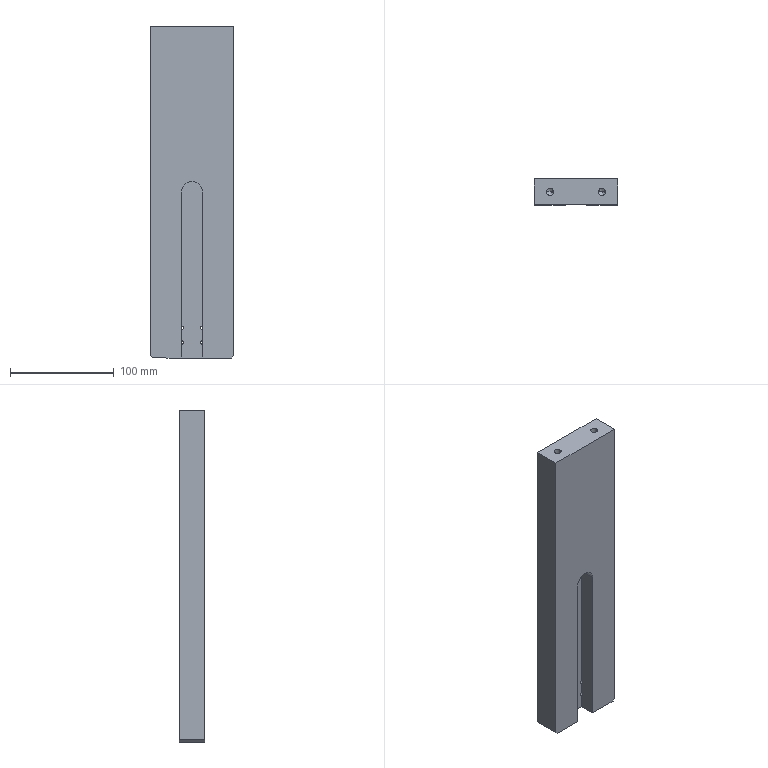Part | SolidWorks | features HoleWzd 3, ICE 3, Chamfer 1, Extrusion 1 | 1 solid | 40 faces | box 80 x 25 x 320 mm | volume 584909 mm3 | cylinder 17 | cone 12 | plane 11 | commonest cylinder face diameters 3.3 x8 6.8 x8 20.5 x1
STEP:
#1=CARTESIAN_POINT('',(18.4,0.,-300.25));
#2=VERTEX_POINT('',#1);
#3=CARTESIAN_POINT('',(11.6,0.,-300.25));
#4=VERTEX_POINT('',#3);
#5=CARTESIAN_POINT('',(15.,0.,-300.25));
#6=DIRECTION('',(0.,0.,-1.));
#7=DIRECTION('',(-1.,0.,0.));
#8=AXIS2_PLACEMENT_3D('',#5,#6,#7);
#9=CIRCLE('',#8,3.4);
#10=EDGE_CURVE('',#2,#4,#9,.T.);
#11=ORIENTED_EDGE('',*,*,#10,.F.);
#12=CARTESIAN_POINT('',(18.4,0.,-320.));
#13=VERTEX_POINT('',#12);
#14=CARTESIAN_POINT('',(18.4,0.,-320.));
#15=DIRECTION('',(0.,0.,-1.));
#16=VECTOR('',#15,1000.);
#17=LINE('',#14,#16);
#18=EDGE_CURVE('',#2,#13,#17,.T.);
#19=ORIENTED_EDGE('',*,*,#18,.T.);
#20=CARTESIAN_POINT('',(11.6,0.,-320.));
#21=VERTEX_POINT('',#20);
#22=CARTESIAN_POINT('',(15.,0.,-320.));
#23=DIRECTION('',(0.,0.,-1.));
#24=DIRECTION('',(-1.,0.,0.));
#25=AXIS2_PLACEMENT_3D('',#22,#23,#24);
#26=CIRCLE('',#25,3.4);
#27=EDGE_CURVE('',#13,#21,#26,.T.);
#28=ORIENTED_EDGE('',*,*,#27,.T.);
#29=CARTESIAN_POINT('',(11.6,0.,-320.));
#30=DIRECTION('',(0.,0.,-1.));
#31=VECTOR('',#30,1000.);
#32=LINE('',#29,#31);
#33=EDGE_CURVE('',#4,#21,#32,.T.);
#34=ORIENTED_EDGE('',*,*,#33,.F.);
#35=EDGE_LOOP('',(#11,#19,#28,#34));
#36=FACE_OUTER_BOUND('',#35,.T.);
#37=CARTESIAN_POINT('',(15.,0.,-320.));
#38=DIRECTION('',(0.,0.,-1.));
#39=DIRECTION('',(-1.,0.,0.));
#40=AXIS2_PLACEMENT_3D('',#37,#38,#39);
#41=CYLINDRICAL_SURFACE('',#40,3.4);
#42=ADVANCED_FACE('',(#36),#41,.F.);
#43=CARTESIAN_POINT('',(15.,0.,-298.207));
#44=VERTEX_POINT('',#43);
#45=CARTESIAN_POINT('',(11.6,0.,-300.25));
#46=DIRECTION('',(-0.8572,0.,-0.515));
#47=VECTOR('',#46,1000.);
#48=LINE('',#45,#47);
#49=EDGE_CURVE('',#44,#4,#48,.T.);
#50=ORIENTED_EDGE('',*,*,#49,.F.);
#51=CARTESIAN_POINT('',(18.4,0.,-300.25));
#52=DIRECTION('',(0.8572,0.,-0.515));
#53=VECTOR('',#52,1000.);
#54=LINE('',#51,#53);
#55=EDGE_CURVE('',#44,#2,#54,.T.);
#56=ORIENTED_EDGE('',*,*,#55,.T.);
#57=ORIENTED_EDGE('',*,*,#10,.T.);
#58=EDGE_LOOP('',(#50,#56,#57));
#59=FACE_OUTER_BOUND('',#58,.T.);
#60=CARTESIAN_POINT('',(15.,0.,-300.25));
#61=DIRECTION('',(0.,0.,-1.));
#62=DIRECTION('',(-1.,0.,0.));
#63=AXIS2_PLACEMENT_3D('',#60,#61,#62);
#64=CONICAL_SURFACE('',#63,3.4,1.03);
#65=ADVANCED_FACE('',(#59),#64,.F.);
#66=CARTESIAN_POINT('',(68.4,0.,-300.25));
#67=VERTEX_POINT('',#66);
#68=CARTESIAN_POINT('',(61.6,0.,-300.25));
#69=VERTEX_POINT('',#68);
#70=CARTESIAN_POINT('',(65.,0.,-300.25));
#71=DIRECTION('',(0.,0.,-1.));
#72=DIRECTION('',(-1.,0.,0.));
#73=AXIS2_PLACEMENT_3D('',#70,#71,#72);
#74=CIRCLE('',#73,3.4);
#75=EDGE_CURVE('',#67,#69,#74,.T.);
#76=ORIENTED_EDGE('',*,*,#75,.F.);
#77=CARTESIAN_POINT('',(68.4,0.,-320.));
#78=VERTEX_POINT('',#77);
#79=CARTESIAN_POINT('',(68.4,0.,-320.));
#80=DIRECTION('',(0.,0.,-1.));
#81=VECTOR('',#80,1000.);
#82=LINE('',#79,#81);
#83=EDGE_CURVE('',#67,#78,#82,.T.);
#84=ORIENTED_EDGE('',*,*,#83,.T.);
#85=CARTESIAN_POINT('',(61.6,0.,-320.));
#86=VERTEX_POINT('',#85);
#87=CARTESIAN_POINT('',(65.,0.,-320.));
#88=DIRECTION('',(0.,0.,-1.));
#89=DIRECTION('',(-1.,0.,0.));
#90=AXIS2_PLACEMENT_3D('',#87,#88,#89);
#91=CIRCLE('',#90,3.4);
#92=EDGE_CURVE('',#78,#86,#91,.T.);
#93=ORIENTED_EDGE('',*,*,#92,.T.);
#94=CARTESIAN_POINT('',(61.6,0.,-320.));
#95=DIRECTION('',(0.,0.,-1.));
#96=VECTOR('',#95,1000.);
#97=LINE('',#94,#96);
#98=EDGE_CURVE('',#69,#86,#97,.T.);
#99=ORIENTED_EDGE('',*,*,#98,.F.);
#100=EDGE_LOOP('',(#76,#84,#93,#99));
#101=FACE_OUTER_BOUND('',#100,.T.);
#102=CARTESIAN_POINT('',(65.,0.,-320.));
#103=DIRECTION('',(0.,0.,-1.));
#104=DIRECTION('',(-1.,0.,0.));
#105=AXIS2_PLACEMENT_3D('',#102,#103,#104);
#106=CYLINDRICAL_SURFACE('',#105,3.4);
#107=ADVANCED_FACE('',(#101),#106,.F.);
#108=CARTESIAN_POINT('',(65.,0.,-298.207));
#109=VERTEX_POINT('',#108);
#110=CARTESIAN_POINT('',(61.6,0.,-300.25));
#111=DIRECTION('',(-0.8572,0.,-0.515));
#112=VECTOR('',#111,1000.);
#113=LINE('',#110,#112);
#114=EDGE_CURVE('',#109,#69,#113,.T.);
#115=ORIENTED_EDGE('',*,*,#114,.F.);
#116=CARTESIAN_POINT('',(68.4,0.,-300.25));
#117=DIRECTION('',(0.8572,0.,-0.515));
#118=VECTOR('',#117,1000.);
#119=LINE('',#116,#118);
#120=EDGE_CURVE('',#109,#67,#119,.T.);
#121=ORIENTED_EDGE('',*,*,#120,.T.);
#122=ORIENTED_EDGE('',*,*,#75,.T.);
#123=EDGE_LOOP('',(#115,#121,#122));
#124=FACE_OUTER_BOUND('',#123,.T.);
#125=CARTESIAN_POINT('',(65.,0.,-300.25));
#126=DIRECTION('',(0.,0.,-1.));
#127=DIRECTION('',(-1.,0.,0.));
#128=AXIS2_PLACEMENT_3D('',#125,#126,#127);
#129=CONICAL_SURFACE('',#128,3.4,1.03);
#130=ADVANCED_FACE('',(#124),#129,.F.);
#131=CARTESIAN_POINT('',(30.,2.5,-306.65));
#132=VERTEX_POINT('',#131);
#133=CARTESIAN_POINT('',(29.75,2.5,-306.631));
#134=VERTEX_POINT('',#133);
#135=CARTESIAN_POINT('',(30.,2.5,-305.));
#136=DIRECTION('',(0.,1.,0.));
#137=DIRECTION('',(0.,0.,-1.));
#138=AXIS2_PLACEMENT_3D('',#135,#136,#137);
#139=CIRCLE('',#138,1.65);
#140=EDGE_CURVE('',#132,#134,#139,.T.);
#141=ORIENTED_EDGE('',*,*,#140,.F.);
#142=CARTESIAN_POINT('',(30.,12.5,-306.65));
#143=VERTEX_POINT('',#142);
#144=CARTESIAN_POINT('',(30.,12.5,-306.65));
#145=DIRECTION('',(0.,1.,0.));
#146=VECTOR('',#145,1000.);
#147=LINE('',#144,#146);
#148=EDGE_CURVE('',#132,#143,#147,.T.);
#149=ORIENTED_EDGE('',*,*,#148,.T.);
#150=CARTESIAN_POINT('',(30.,12.5,-303.35));
#151=VERTEX_POINT('',#150);
#152=CARTESIAN_POINT('',(30.,12.5,-305.));
#153=DIRECTION('',(0.,1.,0.));
#154=DIRECTION('',(0.,0.,1.));
#155=AXIS2_PLACEMENT_3D('',#152,#153,#154);
#156=CIRCLE('',#155,1.65);
#157=EDGE_CURVE('',#143,#151,#156,.T.);
#158=ORIENTED_EDGE('',*,*,#157,.T.);
#159=CARTESIAN_POINT('',(30.,2.5,-303.35));
#160=VERTEX_POINT('',#159);
#161=CARTESIAN_POINT('',(30.,12.5,-303.35));
#162=DIRECTION('',(0.,1.,0.));
#163=VECTOR('',#162,1000.);
#164=LINE('',#161,#163);
#165=EDGE_CURVE('',#160,#151,#164,.T.);
#166=ORIENTED_EDGE('',*,*,#165,.F.);
#167=CARTESIAN_POINT('',(29.75,2.5,-303.369));
#168=VERTEX_POINT('',#167);
#169=CARTESIAN_POINT('',(30.,2.5,-305.));
#170=DIRECTION('',(0.,1.,0.));
#171=DIRECTION('',(0.,0.,-1.));
#172=AXIS2_PLACEMENT_3D('',#169,#170,#171);
#173=CIRCLE('',#172,1.65);
#174=EDGE_CURVE('',#168,#160,#173,.T.);
#175=ORIENTED_EDGE('',*,*,#174,.F.);
#176=CARTESIAN_POINT('',(29.75,2.4,-303.369));
#177=VERTEX_POINT('',#176);
#178=CARTESIAN_POINT('',(29.75,12.5,-303.369));
#179=DIRECTION('',(0.,-1.,0.));
#180=VECTOR('',#179,1000.);
#181=LINE('',#178,#180);
#182=EDGE_CURVE('',#168,#177,#181,.T.);
#183=ORIENTED_EDGE('',*,*,#182,.T.);
#184=CARTESIAN_POINT('',(29.75,2.4,-306.631));
#185=VERTEX_POINT('',#184);
#186=CARTESIAN_POINT('',(30.,2.4,-305.));
#187=DIRECTION('',(0.,1.,0.));
#188=DIRECTION('',(0.,0.,1.));
#189=AXIS2_PLACEMENT_3D('',#186,#187,#188);
#190=CIRCLE('',#189,1.65);
#191=EDGE_CURVE('',#185,#177,#190,.T.);
#192=ORIENTED_EDGE('',*,*,#191,.F.);
#193=CARTESIAN_POINT('',(29.75,12.5,-306.631));
#194=DIRECTION('',(0.,1.,0.));
#195=VECTOR('',#194,1000.);
#196=LINE('',#193,#195);
#197=EDGE_CURVE('',#185,#134,#196,.T.);
#198=ORIENTED_EDGE('',*,*,#197,.T.);
#199=EDGE_LOOP('',(#141,#149,#158,#166,#175,#183,#192,#198));
#200=FACE_OUTER_BOUND('',#199,.T.);
#201=CARTESIAN_POINT('',(30.,12.5,-305.));
#202=DIRECTION('',(0.,1.,0.));
#203=DIRECTION('',(0.,0.,1.));
#204=AXIS2_PLACEMENT_3D('',#201,#202,#203);
#205=CYLINDRICAL_SURFACE('',#204,1.65);
#206=ADVANCED_FACE('',(#200),#205,.F.);
#207=CARTESIAN_POINT('',(30.,2.5,-292.65));
#208=VERTEX_POINT('',#207);
#209=CARTESIAN_POINT('',(29.75,2.5,-292.631));
#210=VERTEX_POINT('',#209);
#211=CARTESIAN_POINT('',(30.,2.5,-291.));
#212=DIRECTION('',(0.,1.,0.));
#213=DIRECTION('',(0.,0.,-1.));
#214=AXIS2_PLACEMENT_3D('',#211,#212,#213);
#215=CIRCLE('',#214,1.65);
#216=EDGE_CURVE('',#208,#210,#215,.T.);
#217=ORIENTED_EDGE('',*,*,#216,.F.);
#218=CARTESIAN_POINT('',(30.,12.5,-292.65));
#219=VERTEX_POINT('',#218);
#220=CARTESIAN_POINT('',(30.,12.5,-292.65));
#221=DIRECTION('',(0.,1.,0.));
#222=VECTOR('',#221,1000.);
#223=LINE('',#220,#222);
#224=EDGE_CURVE('',#208,#219,#223,.T.);
#225=ORIENTED_EDGE('',*,*,#224,.T.);
#226=CARTESIAN_POINT('',(30.,12.5,-289.35));
#227=VERTEX_POINT('',#226);
#228=CARTESIAN_POINT('',(30.,12.5,-291.));
#229=DIRECTION('',(0.,1.,0.));
#230=DIRECTION('',(0.,0.,1.));
#231=AXIS2_PLACEMENT_3D('',#228,#229,#230);
#232=CIRCLE('',#231,1.65);
#233=EDGE_CURVE('',#219,#227,#232,.T.);
#234=ORIENTED_EDGE('',*,*,#233,.T.);
#235=CARTESIAN_POINT('',(30.,2.5,-289.35));
#236=VERTEX_POINT('',#235);
#237=CARTESIAN_POINT('',(30.,12.5,-289.35));
#238=DIRECTION('',(0.,1.,0.));
#239=VECTOR('',#238,1000.);
#240=LINE('',#237,#239);
#241=EDGE_CURVE('',#236,#227,#240,.T.);
#242=ORIENTED_EDGE('',*,*,#241,.F.);
#243=CARTESIAN_POINT('',(29.75,2.5,-289.369));
#244=VERTEX_POINT('',#243);
#245=CARTESIAN_POINT('',(30.,2.5,-291.));
#246=DIRECTION('',(0.,1.,0.));
#247=DIRECTION('',(0.,0.,-1.));
#248=AXIS2_PLACEMENT_3D('',#245,#246,#247);
#249=CIRCLE('',#248,1.65);
#250=EDGE_CURVE('',#244,#236,#249,.T.);
#251=ORIENTED_EDGE('',*,*,#250,.F.);
#252=CARTESIAN_POINT('',(29.75,2.4,-289.369));
#253=VERTEX_POINT('',#252);
#254=CARTESIAN_POINT('',(29.75,12.5,-289.369));
#255=DIRECTION('',(0.,-1.,0.));
#256=VECTOR('',#255,1000.);
#257=LINE('',#254,#256);
#258=EDGE_CURVE('',#244,#253,#257,.T.);
#259=ORIENTED_EDGE('',*,*,#258,.T.);
#260=CARTESIAN_POINT('',(29.75,2.4,-292.631));
#261=VERTEX_POINT('',#260);
#262=CARTESIAN_POINT('',(30.,2.4,-291.));
#263=DIRECTION('',(0.,1.,0.));
#264=DIRECTION('',(0.,0.,1.));
#265=AXIS2_PLACEMENT_3D('',#262,#263,#264);
#266=CIRCLE('',#265,1.65);
#267=EDGE_CURVE('',#261,#253,#266,.T.);
#268=ORIENTED_EDGE('',*,*,#267,.F.);
#269=CARTESIAN_POINT('',(29.75,12.5,-292.631));
#270=DIRECTION('',(0.,1.,0.));
#271=VECTOR('',#270,1000.);
#272=LINE('',#269,#271);
#273=EDGE_CURVE('',#261,#210,#272,.T.);
#274=ORIENTED_EDGE('',*,*,#273,.T.);
#275=EDGE_LOOP('',(#217,#225,#234,#242,#251,#259,#268,#274));
#276=FACE_OUTER_BOUND('',#275,.T.);
#277=CARTESIAN_POINT('',(30.,12.5,-291.));
#278=DIRECTION('',(0.,1.,0.));
#279=DIRECTION('',(0.,0.,1.));
#280=AXIS2_PLACEMENT_3D('',#277,#278,#279);
#281=CYLINDRICAL_SURFACE('',#280,1.65);
#282=ADVANCED_FACE('',(#276),#281,.F.);
#283=CARTESIAN_POINT('',(50.,2.5,-292.65));
#284=VERTEX_POINT('',#283);
#285=CARTESIAN_POINT('',(50.,2.5,-289.35));
#286=VERTEX_POINT('',#285);
#287=CARTESIAN_POINT('',(50.,2.5,-291.));
#288=DIRECTION('',(0.,1.,0.));
#289=DIRECTION('',(0.,0.,-1.));
#290=AXIS2_PLACEMENT_3D('',#287,#288,#289);
#291=CIRCLE('',#290,1.65);
#292=EDGE_CURVE('',#284,#286,#291,.T.);
#293=ORIENTED_EDGE('',*,*,#292,.F.);
#294=CARTESIAN_POINT('',(50.,12.5,-292.65));
#295=VERTEX_POINT('',#294);
#296=CARTESIAN_POINT('',(50.,12.5,-292.65));
#297=DIRECTION('',(0.,1.,0.));
#298=VECTOR('',#297,1000.);
#299=LINE('',#296,#298);
#300=EDGE_CURVE('',#284,#295,#299,.T.);
#301=ORIENTED_EDGE('',*,*,#300,.T.);
#302=CARTESIAN_POINT('',(50.,12.5,-289.35));
#303=VERTEX_POINT('',#302);
#304=CARTESIAN_POINT('',(50.,12.5,-291.));
#305=DIRECTION('',(0.,1.,0.));
#306=DIRECTION('',(0.,0.,1.));
#307=AXIS2_PLACEMENT_3D('',#304,#305,#306);
#308=CIRCLE('',#307,1.65);
#309=EDGE_CURVE('',#295,#303,#308,.T.);
#310=ORIENTED_EDGE('',*,*,#309,.T.);
#311=CARTESIAN_POINT('',(50.,12.5,-289.35));
#312=DIRECTION('',(0.,1.,0.));
#313=VECTOR('',#312,1000.);
#314=LINE('',#311,#313);
#315=EDGE_CURVE('',#286,#303,#314,.T.);
#316=ORIENTED_EDGE('',*,*,#315,.F.);
#317=EDGE_LOOP('',(#293,#301,#310,#316));
#318=FACE_OUTER_BOUND('',#317,.T.);
#319=CARTESIAN_POINT('',(50.,12.5,-291.));
#320=DIRECTION('',(0.,1.,0.));
#321=DIRECTION('',(0.,0.,1.));
#322=AXIS2_PLACEMENT_3D('',#319,#320,#321);
#323=CYLINDRICAL_SURFACE('',#322,1.65);
#324=ADVANCED_FACE('',(#318),#323,.F.);
#325=CARTESIAN_POINT('',(50.,2.5,-306.65));
#326=VERTEX_POINT('',#325);
#327=CARTESIAN_POINT('',(50.,2.5,-303.35));
#328=VERTEX_POINT('',#327);
#329=CARTESIAN_POINT('',(50.,2.5,-305.));
#330=DIRECTION('',(0.,1.,0.));
#331=DIRECTION('',(0.,0.,-1.));
#332=AXIS2_PLACEMENT_3D('',#329,#330,#331);
#333=CIRCLE('',#332,1.65);
#334=EDGE_CURVE('',#326,#328,#333,.T.);
#335=ORIENTED_EDGE('',*,*,#334,.F.);
#336=CARTESIAN_POINT('',(50.,12.5,-306.65));
#337=VERTEX_POINT('',#336);
#338=CARTESIAN_POINT('',(50.,12.5,-306.65));
#339=DIRECTION('',(0.,1.,0.));
#340=VECTOR('',#339,1000.);
#341=LINE('',#338,#340);
#342=EDGE_CURVE('',#326,#337,#341,.T.);
#343=ORIENTED_EDGE('',*,*,#342,.T.);
#344=CARTESIAN_POINT('',(50.,12.5,-303.35));
#345=VERTEX_POINT('',#344);
#346=CARTESIAN_POINT('',(50.,12.5,-305.));
#347=DIRECTION('',(0.,1.,0.));
#348=DIRECTION('',(0.,0.,1.));
#349=AXIS2_PLACEMENT_3D('',#346,#347,#348);
#350=CIRCLE('',#349,1.65);
#351=EDGE_CURVE('',#337,#345,#350,.T.);
#352=ORIENTED_EDGE('',*,*,#351,.T.);
#353=CARTESIAN_POINT('',(50.,12.5,-303.35));
#354=DIRECTION('',(0.,1.,0.));
#355=VECTOR('',#354,1000.);
#356=LINE('',#353,#355);
#357=EDGE_CURVE('',#328,#345,#356,.T.);
#358=ORIENTED_EDGE('',*,*,#357,.F.);
#359=EDGE_LOOP('',(#335,#343,#352,#358));
#360=FACE_OUTER_BOUND('',#359,.T.);
#361=CARTESIAN_POINT('',(50.,12.5,-305.));
#362=DIRECTION('',(0.,1.,0.));
#363=DIRECTION('',(0.,0.,1.));
#364=AXIS2_PLACEMENT_3D('',#361,#362,#363);
#365=CYLINDRICAL_SURFACE('',#364,1.65);
#366=ADVANCED_FACE('',(#360),#365,.F.);
#367=CARTESIAN_POINT('',(11.6,0.,-19.75));
#368=VERTEX_POINT('',#367);
#369=CARTESIAN_POINT('',(18.4,0.,-19.75));
#370=VERTEX_POINT('',#369);
#371=CARTESIAN_POINT('',(15.,0.,-19.75));
#372=DIRECTION('',(0.,0.,1.));
#373=DIRECTION('',(1.,0.,0.));
#374=AXIS2_PLACEMENT_3D('',#371,#372,#373);
#375=CIRCLE('',#374,3.4);
#376=EDGE_CURVE('',#368,#370,#375,.T.);
#377=ORIENTED_EDGE('',*,*,#376,.F.);
#378=CARTESIAN_POINT('',(11.6,0.,0.));
#379=VERTEX_POINT('',#378);
#380=CARTESIAN_POINT('',(11.6,0.,0.));
#381=DIRECTION('',(0.,0.,1.));
#382=VECTOR('',#381,1000.);
#383=LINE('',#380,#382);
#384=EDGE_CURVE('',#368,#379,#383,.T.);
#385=ORIENTED_EDGE('',*,*,#384,.T.);
#386=CARTESIAN_POINT('',(18.4,0.,0.));
#387=VERTEX_POINT('',#386);
#388=CARTESIAN_POINT('',(15.,0.,0.));
#389=DIRECTION('',(0.,0.,1.));
#390=DIRECTION('',(1.,0.,0.));
#391=AXIS2_PLACEMENT_3D('',#388,#389,#390);
#392=CIRCLE('',#391,3.4);
#393=EDGE_CURVE('',#379,#387,#392,.T.);
#394=ORIENTED_EDGE('',*,*,#393,.T.);
#395=CARTESIAN_POINT('',(18.4,0.,0.));
#396=DIRECTION('',(0.,0.,1.));
#397=VECTOR('',#396,1000.);
#398=LINE('',#395,#397);
#399=EDGE_CURVE('',#370,#387,#398,.T.);
#400=ORIENTED_EDGE('',*,*,#399,.F.);
#401=EDGE_LOOP('',(#377,#385,#394,#400));
#402=FACE_OUTER_BOUND('',#401,.T.);
#403=CARTESIAN_POINT('',(15.,0.,0.));
#404=DIRECTION('',(0.,0.,1.));
#405=DIRECTION('',(1.,0.,0.));
#406=AXIS2_PLACEMENT_3D('',#403,#404,#405);
#407=CYLINDRICAL_SURFACE('',#406,3.4);
#408=ADVANCED_FACE('',(#402),#407,.F.);
#409=CARTESIAN_POINT('',(15.,0.,-21.793));
#410=VERTEX_POINT('',#409);
#411=CARTESIAN_POINT('',(18.4,0.,-19.75));
#412=DIRECTION('',(0.8572,0.,0.515));
#413=VECTOR('',#412,1000.);
#414=LINE('',#411,#413);
#415=EDGE_CURVE('',#410,#370,#414,.T.);
#416=ORIENTED_EDGE('',*,*,#415,.F.);
#417=CARTESIAN_POINT('',(11.6,0.,-19.75));
#418=DIRECTION('',(-0.8572,0.,0.515));
#419=VECTOR('',#418,1000.);
#420=LINE('',#417,#419);
#421=EDGE_CURVE('',#410,#368,#420,.T.);
#422=ORIENTED_EDGE('',*,*,#421,.T.);
#423=ORIENTED_EDGE('',*,*,#376,.T.);
#424=EDGE_LOOP('',(#416,#422,#423));
#425=FACE_OUTER_BOUND('',#424,.T.);
#426=CARTESIAN_POINT('',(15.,0.,-19.75));
#427=DIRECTION('',(0.,0.,1.));
#428=DIRECTION('',(1.,0.,0.));
#429=AXIS2_PLACEMENT_3D('',#426,#427,#428);
#430=CONICAL_SURFACE('',#429,3.4,1.03);
#431=ADVANCED_FACE('',(#425),#430,.F.);
#432=CARTESIAN_POINT('',(61.6,0.,-19.75));
#433=VERTEX_POINT('',#432);
#434=CARTESIAN_POINT('',(68.4,0.,-19.75));
#435=VERTEX_POINT('',#434);
#436=CARTESIAN_POINT('',(65.,0.,-19.75));
#437=DIRECTION('',(0.,0.,1.));
#438=DIRECTION('',(1.,0.,0.));
#439=AXIS2_PLACEMENT_3D('',#436,#437,#438);
#440=CIRCLE('',#439,3.4);
#441=EDGE_CURVE('',#433,#435,#440,.T.);
#442=ORIENTED_EDGE('',*,*,#441,.F.);
#443=CARTESIAN_POINT('',(61.6,0.,0.));
#444=VERTEX_POINT('',#443);
#445=CARTESIAN_POINT('',(61.6,0.,0.));
#446=DIRECTION('',(0.,0.,1.));
#447=VECTOR('',#446,1000.);
#448=LINE('',#445,#447);
#449=EDGE_CURVE('',#433,#444,#448,.T.);
#450=ORIENTED_EDGE('',*,*,#449,.T.);
#451=CARTESIAN_POINT('',(68.4,0.,0.));
#452=VERTEX_POINT('',#451);
#453=CARTESIAN_POINT('',(65.,0.,0.));
#454=DIRECTION('',(0.,0.,1.));
#455=DIRECTION('',(1.,0.,0.));
#456=AXIS2_PLACEMENT_3D('',#453,#454,#455);
#457=CIRCLE('',#456,3.4);
#458=EDGE_CURVE('',#444,#452,#457,.T.);
#459=ORIENTED_EDGE('',*,*,#458,.T.);
#460=CARTESIAN_POINT('',(68.4,0.,0.));
#461=DIRECTION('',(0.,0.,1.));
#462=VECTOR('',#461,1000.);
#463=LINE('',#460,#462);
#464=EDGE_CURVE('',#435,#452,#463,.T.);
#465=ORIENTED_EDGE('',*,*,#464,.F.);
#466=EDGE_LOOP('',(#442,#450,#459,#465));
#467=FACE_OUTER_BOUND('',#466,.T.);
#468=CARTESIAN_POINT('',(65.,0.,0.));
#469=DIRECTION('',(0.,0.,1.));
#470=DIRECTION('',(1.,0.,0.));
#471=AXIS2_PLACEMENT_3D('',#468,#469,#470);
#472=CYLINDRICAL_SURFACE('',#471,3.4);
#473=ADVANCED_FACE('',(#467),#472,.F.);
#474=CARTESIAN_POINT('',(65.,0.,-21.793));
#475=VERTEX_POINT('',#474);
#476=CARTESIAN_POINT('',(68.4,0.,-19.75));
#477=DIRECTION('',(0.8572,0.,0.515));
#478=VECTOR('',#477,1000.);
#479=LINE('',#476,#478);
#480=EDGE_CURVE('',#475,#435,#479,.T.);
#481=ORIENTED_EDGE('',*,*,#480,.F.);
#482=CARTESIAN_POINT('',(61.6,0.,-19.75));
#483=DIRECTION('',(-0.8572,0.,0.515));
#484=VECTOR('',#483,1000.);
#485=LINE('',#482,#484);
#486=EDGE_CURVE('',#475,#433,#485,.T.);
#487=ORIENTED_EDGE('',*,*,#486,.T.);
#488=ORIENTED_EDGE('',*,*,#441,.T.);
#489=EDGE_LOOP('',(#481,#487,#488));
#490=FACE_OUTER_BOUND('',#489,.T.);
#491=CARTESIAN_POINT('',(65.,0.,-19.75));
#492=DIRECTION('',(0.,0.,1.));
#493=DIRECTION('',(1.,0.,0.));
#494=AXIS2_PLACEMENT_3D('',#491,#492,#493);
#495=CONICAL_SURFACE('',#494,3.4,1.03);
#496=ADVANCED_FACE('',(#490),#495,.F.);
#497=CARTESIAN_POINT('',(15.,0.,0.));
#498=DIRECTION('',(0.,0.,1.));
#499=DIRECTION('',(1.,0.,0.));
#500=AXIS2_PLACEMENT_3D('',#497,#498,#499);
#501=CIRCLE('',#500,3.4);
#502=EDGE_CURVE('',#387,#379,#501,.T.);
#503=ORIENTED_EDGE('',*,*,#502,.F.);
#504=ORIENTED_EDGE('',*,*,#393,.F.);
#505=EDGE_LOOP('',(#503,#504));
#506=FACE_BOUND('',#505,.T.);
#507=CARTESIAN_POINT('',(65.,0.,0.));
#508=DIRECTION('',(0.,0.,1.));
#509=DIRECTION('',(1.,0.,0.));
#510=AXIS2_PLACEMENT_3D('',#507,#508,#509);
#511=CIRCLE('',#510,3.4);
#512=EDGE_CURVE('',#452,#444,#511,.T.);
#513=ORIENTED_EDGE('',*,*,#512,.F.);
#514=ORIENTED_EDGE('',*,*,#458,.F.);
#515=EDGE_LOOP('',(#513,#514));
#516=FACE_BOUND('',#515,.T.);
#517=CARTESIAN_POINT('',(0.,-12.5,0.));
#518=VERTEX_POINT('',#517);
#519=CARTESIAN_POINT('',(80.,-12.5,0.));
#520=VERTEX_POINT('',#519);
#521=CARTESIAN_POINT('',(0.,-12.5,0.));
#522=DIRECTION('',(1.,0.,0.));
#523=VECTOR('',#522,1000.);
#524=LINE('',#521,#523);
#525=EDGE_CURVE('',#518,#520,#524,.T.);
#526=ORIENTED_EDGE('',*,*,#525,.T.);
#527=CARTESIAN_POINT('',(80.,12.5,0.));
#528=VERTEX_POINT('',#527);
#529=CARTESIAN_POINT('',(80.,12.5,0.));
#530=DIRECTION('',(0.,-1.,0.));
#531=VECTOR('',#530,1000.);
#532=LINE('',#529,#531);
#533=EDGE_CURVE('',#528,#520,#532,.T.);
#534=ORIENTED_EDGE('',*,*,#533,.F.);
#535=CARTESIAN_POINT('',(0.,12.5,0.));
#536=VERTEX_POINT('',#535);
#537=CARTESIAN_POINT('',(0.,12.5,0.));
#538=DIRECTION('',(1.,0.,0.));
#539=VECTOR('',#538,1000.);
#540=LINE('',#537,#539);
#541=EDGE_CURVE('',#536,#528,#540,.T.);
#542=ORIENTED_EDGE('',*,*,#541,.F.);
#543=CARTESIAN_POINT('',(0.,12.5,0.));
#544=DIRECTION('',(0.,-1.,0.));
#545=VECTOR('',#544,1000.);
#546=LINE('',#543,#545);
#547=EDGE_CURVE('',#536,#518,#546,.T.);
#548=ORIENTED_EDGE('',*,*,#547,.T.);
#549=EDGE_LOOP('',(#526,#534,#542,#548));
#550=FACE_OUTER_BOUND('',#549,.T.);
#551=CARTESIAN_POINT('',(0.,12.5,0.));
#552=DIRECTION('',(0.,0.,-1.));
#553=DIRECTION('',(-1.,0.,0.));
#554=AXIS2_PLACEMENT_3D('',#551,#552,#553);
#555=PLANE('',#554);
#556=ADVANCED_FACE('',(#506,#516,#550),#555,.F.);
#557=CARTESIAN_POINT('',(80.,-12.5,-318.));
#558=VERTEX_POINT('',#557);
#559=CARTESIAN_POINT('',(80.,-12.5,0.));
#560=DIRECTION('',(0.,0.,-1.));
#561=VECTOR('',#560,1000.);
#562=LINE('',#559,#561);
#563=EDGE_CURVE('',#520,#558,#562,.T.);
#564=ORIENTED_EDGE('',*,*,#563,.T.);
#565=CARTESIAN_POINT('',(80.,12.5,-318.));
#566=VERTEX_POINT('',#565);
#567=CARTESIAN_POINT('',(80.,12.5,-318.));
#568=DIRECTION('',(0.,1.,0.));
#569=VECTOR('',#568,1000.);
#570=LINE('',#567,#569);
#571=EDGE_CURVE('',#558,#566,#570,.T.);
#572=ORIENTED_EDGE('',*,*,#571,.T.);
#573=CARTESIAN_POINT('',(80.,12.5,0.));
#574=DIRECTION('',(0.,0.,-1.));
#575=VECTOR('',#574,1000.);
#576=LINE('',#573,#575);
#577=EDGE_CURVE('',#528,#566,#576,.T.);
#578=ORIENTED_EDGE('',*,*,#577,.F.);
#579=ORIENTED_EDGE('',*,*,#533,.T.);
#580=EDGE_LOOP('',(#564,#572,#578,#579));
#581=FACE_OUTER_BOUND('',#580,.T.);
#582=CARTESIAN_POINT('',(80.,12.5,0.));
#583=DIRECTION('',(-1.,0.,0.));
#584=DIRECTION('',(0.,0.,1.));
#585=AXIS2_PLACEMENT_3D('',#582,#583,#584);
#586=PLANE('',#585);
#587=ADVANCED_FACE('',(#581),#586,.F.);
#588=CARTESIAN_POINT('',(78.,-12.5,-320.));
#589=VERTEX_POINT('',#588);
#590=CARTESIAN_POINT('',(50.25,-12.5,-320.));
#591=VERTEX_POINT('',#590);
#592=CARTESIAN_POINT('',(80.,-12.5,-320.));
#593=DIRECTION('',(-1.,0.,0.));
#594=VECTOR('',#593,1000.);
#595=LINE('',#592,#594);
#596=EDGE_CURVE('',#589,#591,#595,.T.);
#597=ORIENTED_EDGE('',*,*,#596,.T.);
#598=CARTESIAN_POINT('',(50.25,2.5,-320.));
#599=VERTEX_POINT('',#598);
#600=CARTESIAN_POINT('',(50.25,2.5,-320.));
#601=DIRECTION('',(0.,-1.,0.));
#602=VECTOR('',#601,1000.);
#603=LINE('',#600,#602);
#604=EDGE_CURVE('',#599,#591,#603,.T.);
#605=ORIENTED_EDGE('',*,*,#604,.F.);
#606=CARTESIAN_POINT('',(29.75,2.5,-320.));
#607=VERTEX_POINT('',#606);
#608=CARTESIAN_POINT('',(80.,2.5,-320.));
#609=DIRECTION('',(1.,0.,0.));
#610=VECTOR('',#609,1000.);
#611=LINE('',#608,#610);
#612=EDGE_CURVE('',#607,#599,#611,.T.);
#613=ORIENTED_EDGE('',*,*,#612,.F.);
#614=CARTESIAN_POINT('',(29.75,-12.5,-320.));
#615=VERTEX_POINT('',#614);
#616=CARTESIAN_POINT('',(29.75,2.5,-320.));
#617=DIRECTION('',(0.,-1.,0.));
#618=VECTOR('',#617,1000.);
#619=LINE('',#616,#618);
#620=EDGE_CURVE('',#607,#615,#619,.T.);
#621=ORIENTED_EDGE('',*,*,#620,.T.);
#622=CARTESIAN_POINT('',(2.,-12.5,-320.));
#623=VERTEX_POINT('',#622);
#624=CARTESIAN_POINT('',(80.,-12.5,-320.));
#625=DIRECTION('',(-1.,0.,0.));
#626=VECTOR('',#625,1000.);
#627=LINE('',#624,#626);
#628=EDGE_CURVE('',#615,#623,#627,.T.);
#629=ORIENTED_EDGE('',*,*,#628,.T.);
#630=CARTESIAN_POINT('',(2.,12.5,-320.));
#631=VERTEX_POINT('',#630);
#632=CARTESIAN_POINT('',(2.,12.5,-320.));
#633=DIRECTION('',(0.,1.,0.));
#634=VECTOR('',#633,1000.);
#635=LINE('',#632,#634);
#636=EDGE_CURVE('',#623,#631,#635,.T.);
#637=ORIENTED_EDGE('',*,*,#636,.T.);
#638=CARTESIAN_POINT('',(78.,12.5,-320.));
#639=VERTEX_POINT('',#638);
#640=CARTESIAN_POINT('',(80.,12.5,-320.));
#641=DIRECTION('',(-1.,0.,0.));
#642=VECTOR('',#641,1000.);
#643=LINE('',#640,#642);
#644=EDGE_CURVE('',#639,#631,#643,.T.);
#645=ORIENTED_EDGE('',*,*,#644,.F.);
#646=CARTESIAN_POINT('',(78.,12.5,-320.));
#647=DIRECTION('',(0.,-1.,0.));
#648=VECTOR('',#647,1000.);
#649=LINE('',#646,#648);
#650=EDGE_CURVE('',#639,#589,#649,.T.);
#651=ORIENTED_EDGE('',*,*,#650,.T.);
#652=EDGE_LOOP('',(#597,#605,#613,#621,#629,#637,#645,#651));
#653=FACE_OUTER_BOUND('',#652,.T.);
#654=CARTESIAN_POINT('',(15.,0.,-320.));
#655=DIRECTION('',(0.,0.,-1.));
#656=DIRECTION('',(-1.,0.,0.));
#657=AXIS2_PLACEMENT_3D('',#654,#655,#656);
#658=CIRCLE('',#657,3.4);
#659=EDGE_CURVE('',#21,#13,#658,.T.);
#660=ORIENTED_EDGE('',*,*,#659,.F.);
#661=ORIENTED_EDGE('',*,*,#27,.F.);
#662=EDGE_LOOP('',(#660,#661));
#663=FACE_BOUND('',#662,.T.);
#664=CARTESIAN_POINT('',(65.,0.,-320.));
#665=DIRECTION('',(0.,0.,-1.));
#666=DIRECTION('',(-1.,0.,0.));
#667=AXIS2_PLACEMENT_3D('',#664,#665,#666);
#668=CIRCLE('',#667,3.4);
#669=EDGE_CURVE('',#86,#78,#668,.T.);
#670=ORIENTED_EDGE('',*,*,#669,.F.);
#671=ORIENTED_EDGE('',*,*,#92,.F.);
#672=EDGE_LOOP('',(#670,#671));
#673=FACE_BOUND('',#672,.T.);
#674=CARTESIAN_POINT('',(80.,12.5,-320.));
#675=DIRECTION('',(0.,0.,1.));
#676=DIRECTION('',(1.,0.,0.));
#677=AXIS2_PLACEMENT_3D('',#674,#675,#676);
#678=PLANE('',#677);
#679=ADVANCED_FACE('',(#653,#663,#673),#678,.F.);
#680=CARTESIAN_POINT('',(0.,12.5,-318.));
#681=VERTEX_POINT('',#680);
#682=CARTESIAN_POINT('',(0.,12.5,-320.));
#683=DIRECTION('',(0.,0.,1.));
#684=VECTOR('',#683,1000.);
#685=LINE('',#682,#684);
#686=EDGE_CURVE('',#681,#536,#685,.T.);
#687=ORIENTED_EDGE('',*,*,#686,.F.);
#688=CARTESIAN_POINT('',(0.,-12.5,-318.));
#689=VERTEX_POINT('',#688);
#690=CARTESIAN_POINT('',(0.,12.5,-318.));
#691=DIRECTION('',(0.,-1.,0.));
#692=VECTOR('',#691,1000.);
#693=LINE('',#690,#692);
#694=EDGE_CURVE('',#681,#689,#693,.T.);
#695=ORIENTED_EDGE('',*,*,#694,.T.);
#696=CARTESIAN_POINT('',(0.,-12.5,-320.));
#697=DIRECTION('',(0.,0.,1.));
#698=VECTOR('',#697,1000.);
#699=LINE('',#696,#698);
#700=EDGE_CURVE('',#689,#518,#699,.T.);
#701=ORIENTED_EDGE('',*,*,#700,.T.);
#702=ORIENTED_EDGE('',*,*,#547,.F.);
#703=EDGE_LOOP('',(#687,#695,#701,#702));
#704=FACE_OUTER_BOUND('',#703,.T.);
#705=CARTESIAN_POINT('',(0.,12.5,-320.));
#706=DIRECTION('',(1.,0.,0.));
#707=DIRECTION('',(0.,0.,-1.));
#708=AXIS2_PLACEMENT_3D('',#705,#706,#707);
#709=PLANE('',#708);
#710=ADVANCED_FACE('',(#704),#709,.F.);
#711=CARTESIAN_POINT('',(30.,12.5,-305.));
#712=DIRECTION('',(0.,1.,0.));
#713=DIRECTION('',(0.,0.,1.));
#714=AXIS2_PLACEMENT_3D('',#711,#712,#713);
#715=CIRCLE('',#714,1.65);
#716=EDGE_CURVE('',#151,#143,#715,.T.);
#717=ORIENTED_EDGE('',*,*,#716,.F.);
#718=ORIENTED_EDGE('',*,*,#157,.F.);
#719=EDGE_LOOP('',(#717,#718));
#720=FACE_BOUND('',#719,.T.);
#721=CARTESIAN_POINT('',(30.,12.5,-291.));
#722=DIRECTION('',(0.,1.,0.));
#723=DIRECTION('',(0.,0.,1.));
#724=AXIS2_PLACEMENT_3D('',#721,#722,#723);
#725=CIRCLE('',#724,1.65);
#726=EDGE_CURVE('',#227,#219,#725,.T.);
#727=ORIENTED_EDGE('',*,*,#726,.F.);
#728=ORIENTED_EDGE('',*,*,#233,.F.);
#729=EDGE_LOOP('',(#727,#728));
#730=FACE_BOUND('',#729,.T.);
#731=CARTESIAN_POINT('',(50.,12.5,-291.));
#732=DIRECTION('',(0.,1.,0.));
#733=DIRECTION('',(0.,0.,1.));
#734=AXIS2_PLACEMENT_3D('',#731,#732,#733);
#735=CIRCLE('',#734,1.65);
#736=EDGE_CURVE('',#303,#295,#735,.T.);
#737=ORIENTED_EDGE('',*,*,#736,.F.);
#738=ORIENTED_EDGE('',*,*,#309,.F.);
#739=EDGE_LOOP('',(#737,#738));
#740=FACE_BOUND('',#739,.T.);
#741=CARTESIAN_POINT('',(50.,12.5,-305.));
#742=DIRECTION('',(0.,1.,0.));
#743=DIRECTION('',(0.,0.,1.));
#744=AXIS2_PLACEMENT_3D('',#741,#742,#743);
#745=CIRCLE('',#744,1.65);
#746=EDGE_CURVE('',#345,#337,#745,.T.);
#747=ORIENTED_EDGE('',*,*,#746,.F.);
#748=ORIENTED_EDGE('',*,*,#351,.F.);
#749=EDGE_LOOP('',(#747,#748));
#750=FACE_BOUND('',#749,.T.);
#751=ORIENTED_EDGE('',*,*,#644,.T.);
#752=CARTESIAN_POINT('',(-159.,12.5,-159.));
#753=DIRECTION('',(-0.7071,0.,0.7071));
#754=VECTOR('',#753,1000.);
#755=LINE('',#752,#754);
#756=EDGE_CURVE('',#631,#681,#755,.T.);
#757=ORIENTED_EDGE('',*,*,#756,.T.);
#758=ORIENTED_EDGE('',*,*,#686,.T.);
#759=ORIENTED_EDGE('',*,*,#541,.T.);
#760=ORIENTED_EDGE('',*,*,#577,.T.);
#761=CARTESIAN_POINT('',(199.,12.5,-199.));
#762=DIRECTION('',(-0.7071,0.,-0.7071));
#763=VECTOR('',#762,1000.);
#764=LINE('',#761,#763);
#765=EDGE_CURVE('',#566,#639,#764,.T.);
#766=ORIENTED_EDGE('',*,*,#765,.T.);
#767=EDGE_LOOP('',(#751,#757,#758,#759,#760,#766));
#768=FACE_OUTER_BOUND('',#767,.T.);
#769=CARTESIAN_POINT('',(0.,12.5,0.));
#770=DIRECTION('',(0.,1.,0.));
#771=DIRECTION('',(0.,0.,1.));
#772=AXIS2_PLACEMENT_3D('',#769,#770,#771);
#773=PLANE('',#772);
#774=ADVANCED_FACE('',(#720,#730,#740,#750,#768),#773,.T.);
#775=CARTESIAN_POINT('',(50.25,-12.5,-160.));
#776=VERTEX_POINT('',#775);
#777=CARTESIAN_POINT('',(29.75,-12.5,-160.));
#778=VERTEX_POINT('',#777);
#779=CARTESIAN_POINT('',(40.,-12.5,-160.));
#780=DIRECTION('',(0.,-1.,0.));
#781=DIRECTION('',(0.,0.,-1.));
#782=AXIS2_PLACEMENT_3D('',#779,#780,#781);
#783=CIRCLE('',#782,10.25);
#784=EDGE_CURVE('',#776,#778,#783,.T.);
#785=ORIENTED_EDGE('',*,*,#784,.F.);
#786=CARTESIAN_POINT('',(50.25,-12.5,-160.));
#787=DIRECTION('',(0.,0.,1.));
#788=VECTOR('',#787,1000.);
#789=LINE('',#786,#788);
#790=EDGE_CURVE('',#591,#776,#789,.T.);
#791=ORIENTED_EDGE('',*,*,#790,.F.);
#792=ORIENTED_EDGE('',*,*,#596,.F.);
#793=CARTESIAN_POINT('',(78.,-12.5,-320.));
#794=DIRECTION('',(0.7071,0.,0.7071));
#795=VECTOR('',#794,1000.);
#796=LINE('',#793,#795);
#797=EDGE_CURVE('',#589,#558,#796,.T.);
#798=ORIENTED_EDGE('',*,*,#797,.T.);
#799=ORIENTED_EDGE('',*,*,#563,.F.);
#800=ORIENTED_EDGE('',*,*,#525,.F.);
#801=ORIENTED_EDGE('',*,*,#700,.F.);
#802=CARTESIAN_POINT('',(0.,-12.5,-318.));
#803=DIRECTION('',(0.7071,0.,-0.7071));
#804=VECTOR('',#803,1000.);
#805=LINE('',#802,#804);
#806=EDGE_CURVE('',#689,#623,#805,.T.);
#807=ORIENTED_EDGE('',*,*,#806,.T.);
#808=ORIENTED_EDGE('',*,*,#628,.F.);
#809=CARTESIAN_POINT('',(29.75,-12.5,-160.));
#810=DIRECTION('',(0.,0.,-1.));
#811=VECTOR('',#810,1000.);
#812=LINE('',#809,#811);
#813=EDGE_CURVE('',#778,#615,#812,.T.);
#814=ORIENTED_EDGE('',*,*,#813,.F.);
#815=EDGE_LOOP('',(#785,#791,#792,#798,#799,#800,#801,#807,#808,#814));
#816=FACE_OUTER_BOUND('',#815,.T.);
#817=CARTESIAN_POINT('',(0.,-12.5,0.));
#818=DIRECTION('',(0.,1.,0.));
#819=DIRECTION('',(0.,0.,1.));
#820=AXIS2_PLACEMENT_3D('',#817,#818,#819);
#821=PLANE('',#820);
#822=ADVANCED_FACE('',(#816),#821,.F.);
#823=ORIENTED_EDGE('',*,*,#486,.F.);
#824=ORIENTED_EDGE('',*,*,#480,.T.);
#825=CARTESIAN_POINT('',(65.,0.,-19.75));
#826=DIRECTION('',(0.,0.,1.));
#827=DIRECTION('',(1.,0.,0.));
#828=AXIS2_PLACEMENT_3D('',#825,#826,#827);
#829=CIRCLE('',#828,3.4);
#830=EDGE_CURVE('',#435,#433,#829,.T.);
#831=ORIENTED_EDGE('',*,*,#830,.T.);
#832=EDGE_LOOP('',(#823,#824,#831));
#833=FACE_OUTER_BOUND('',#832,.T.);
#834=CARTESIAN_POINT('',(65.,0.,-19.75));
#835=DIRECTION('',(0.,0.,1.));
#836=DIRECTION('',(1.,0.,0.));
#837=AXIS2_PLACEMENT_3D('',#834,#835,#836);
#838=CONICAL_SURFACE('',#837,3.4,1.03);
#839=ADVANCED_FACE('',(#833),#838,.F.);
#840=ORIENTED_EDGE('',*,*,#449,.F.);
#841=ORIENTED_EDGE('',*,*,#830,.F.);
#842=ORIENTED_EDGE('',*,*,#464,.T.);
#843=ORIENTED_EDGE('',*,*,#512,.T.);
#844=EDGE_LOOP('',(#840,#841,#842,#843));
#845=FACE_OUTER_BOUND('',#844,.T.);
#846=CARTESIAN_POINT('',(65.,0.,0.));
#847=DIRECTION('',(0.,0.,1.));
#848=DIRECTION('',(1.,0.,0.));
#849=AXIS2_PLACEMENT_3D('',#846,#847,#848);
#850=CYLINDRICAL_SURFACE('',#849,3.4);
#851=ADVANCED_FACE('',(#845),#850,.F.);
#852=ORIENTED_EDGE('',*,*,#421,.F.);
#853=ORIENTED_EDGE('',*,*,#415,.T.);
#854=CARTESIAN_POINT('',(15.,0.,-19.75));
#855=DIRECTION('',(0.,0.,1.));
#856=DIRECTION('',(1.,0.,0.));
#857=AXIS2_PLACEMENT_3D('',#854,#855,#856);
#858=CIRCLE('',#857,3.4);
#859=EDGE_CURVE('',#370,#368,#858,.T.);
#860=ORIENTED_EDGE('',*,*,#859,.T.);
#861=EDGE_LOOP('',(#852,#853,#860));
#862=FACE_OUTER_BOUND('',#861,.T.);
#863=CARTESIAN_POINT('',(15.,0.,-19.75));
#864=DIRECTION('',(0.,0.,1.));
#865=DIRECTION('',(1.,0.,0.));
#866=AXIS2_PLACEMENT_3D('',#863,#864,#865);
#867=CONICAL_SURFACE('',#866,3.4,1.03);
#868=ADVANCED_FACE('',(#862),#867,.F.);
#869=ORIENTED_EDGE('',*,*,#384,.F.);
#870=ORIENTED_EDGE('',*,*,#859,.F.);
#871=ORIENTED_EDGE('',*,*,#399,.T.);
#872=ORIENTED_EDGE('',*,*,#502,.T.);
#873=EDGE_LOOP('',(#869,#870,#871,#872));
#874=FACE_OUTER_BOUND('',#873,.T.);
#875=CARTESIAN_POINT('',(15.,0.,0.));
#876=DIRECTION('',(0.,0.,1.));
#877=DIRECTION('',(1.,0.,0.));
#878=AXIS2_PLACEMENT_3D('',#875,#876,#877);
#879=CYLINDRICAL_SURFACE('',#878,3.4);
#880=ADVANCED_FACE('',(#874),#879,.F.);
#881=ORIENTED_EDGE('',*,*,#756,.F.);
#882=ORIENTED_EDGE('',*,*,#636,.F.);
#883=ORIENTED_EDGE('',*,*,#806,.F.);
#884=ORIENTED_EDGE('',*,*,#694,.F.);
#885=EDGE_LOOP('',(#881,#882,#883,#884));
#886=FACE_OUTER_BOUND('',#885,.T.);
#887=CARTESIAN_POINT('',(0.,12.5,-318.));
#888=DIRECTION('',(0.7071,0.,0.7071));
#889=DIRECTION('',(0.,-1.,0.));
#890=AXIS2_PLACEMENT_3D('',#887,#888,#889);
#891=PLANE('',#890);
#892=ADVANCED_FACE('',(#886),#891,.F.);
#893=ORIENTED_EDGE('',*,*,#765,.F.);
#894=ORIENTED_EDGE('',*,*,#571,.F.);
#895=ORIENTED_EDGE('',*,*,#797,.F.);
#896=ORIENTED_EDGE('',*,*,#650,.F.);
#897=EDGE_LOOP('',(#893,#894,#895,#896));
#898=FACE_OUTER_BOUND('',#897,.T.);
#899=CARTESIAN_POINT('',(78.,12.5,-320.));
#900=DIRECTION('',(-0.7071,0.,0.7071));
#901=DIRECTION('',(0.,-1.,0.));
#902=AXIS2_PLACEMENT_3D('',#899,#900,#901);
#903=PLANE('',#902);
#904=ADVANCED_FACE('',(#898),#903,.F.);
#905=CARTESIAN_POINT('',(50.25,2.4,-303.369));
#906=VERTEX_POINT('',#905);
#907=CARTESIAN_POINT('',(50.25,2.4,-306.631));
#908=VERTEX_POINT('',#907);
#909=CARTESIAN_POINT('',(50.,2.4,-305.));
#910=DIRECTION('',(0.,1.,0.));
#911=DIRECTION('',(0.,0.,1.));
#912=AXIS2_PLACEMENT_3D('',#909,#910,#911);
#913=CIRCLE('',#912,1.65);
#914=EDGE_CURVE('',#906,#908,#913,.T.);
#915=ORIENTED_EDGE('',*,*,#914,.T.);
#916=CARTESIAN_POINT('',(50.25,2.4,-306.631));
#917=CARTESIAN_POINT('',(50.25,2.243,-306.366));
#918=CARTESIAN_POINT('',(50.25,2.085,-306.101));
#919=CARTESIAN_POINT('',(50.25,1.855,-305.7));
#920=CARTESIAN_POINT('',(50.25,1.778,-305.566));
#921=CARTESIAN_POINT('',(50.25,1.672,-305.361));
#922=CARTESIAN_POINT('',(50.25,1.637,-305.292));
#923=CARTESIAN_POINT('',(50.25,1.58,-305.149));
#924=CARTESIAN_POINT('',(50.25,1.558,-305.073));
#925=CARTESIAN_POINT('',(50.25,1.559,-304.92));
#926=CARTESIAN_POINT('',(50.25,1.583,-304.845));
#927=CARTESIAN_POINT('',(50.25,1.64,-304.702));
#928=CARTESIAN_POINT('',(50.25,1.675,-304.633));
#929=CARTESIAN_POINT('',(50.25,1.781,-304.429));
#930=CARTESIAN_POINT('',(50.25,1.857,-304.296));
#931=CARTESIAN_POINT('',(50.25,2.087,-303.897));
#932=CARTESIAN_POINT('',(50.25,2.243,-303.633));
#933=CARTESIAN_POINT('',(50.25,2.4,-303.369));
#934=B_SPLINE_CURVE_WITH_KNOTS('',3,(#916,#917,#918,#919,#920,#921,#922,#923,#924,#925,#926,#927,#928,#929,#930,#931,#932,#933),.UNSPECIFIED.,.F.,.F.,(4,2,2,2,2,2,2,2,4),(0.004038,0.004963,0.005426,0.005657,0.005888,0.006119,0.006351,0.006813,0.007738),.UNSPECIFIED.);
#935=EDGE_CURVE('',#908,#906,#934,.T.);
#936=ORIENTED_EDGE('',*,*,#935,.T.);
#937=EDGE_LOOP('',(#915,#936));
#938=FACE_OUTER_BOUND('',#937,.T.);
#939=CARTESIAN_POINT('',(50.,2.4,-305.));
#940=DIRECTION('',(0.,1.,0.));
#941=DIRECTION('',(0.,0.,1.));
#942=AXIS2_PLACEMENT_3D('',#939,#940,#941);
#943=CONICAL_SURFACE('',#942,1.65,1.03);
#944=ADVANCED_FACE('',(#938),#943,.F.);
#945=ORIENTED_EDGE('',*,*,#342,.F.);
#946=CARTESIAN_POINT('',(50.25,2.5,-306.631));
#947=VERTEX_POINT('',#946);
#948=CARTESIAN_POINT('',(50.,2.5,-305.));
#949=DIRECTION('',(0.,1.,0.));
#950=DIRECTION('',(0.,0.,-1.));
#951=AXIS2_PLACEMENT_3D('',#948,#949,#950);
#952=CIRCLE('',#951,1.65);
#953=EDGE_CURVE('',#947,#326,#952,.T.);
#954=ORIENTED_EDGE('',*,*,#953,.F.);
#955=CARTESIAN_POINT('',(50.25,12.5,-306.631));
#956=DIRECTION('',(0.,-1.,0.));
#957=VECTOR('',#956,1000.);
#958=LINE('',#955,#957);
#959=EDGE_CURVE('',#947,#908,#958,.T.);
#960=ORIENTED_EDGE('',*,*,#959,.T.);
#961=ORIENTED_EDGE('',*,*,#914,.F.);
#962=CARTESIAN_POINT('',(50.25,2.5,-303.369));
#963=VERTEX_POINT('',#962);
#964=CARTESIAN_POINT('',(50.25,12.5,-303.369));
#965=DIRECTION('',(0.,1.,0.));
#966=VECTOR('',#965,1000.);
#967=LINE('',#964,#966);
#968=EDGE_CURVE('',#906,#963,#967,.T.);
#969=ORIENTED_EDGE('',*,*,#968,.T.);
#970=CARTESIAN_POINT('',(50.,2.5,-305.));
#971=DIRECTION('',(0.,1.,0.));
#972=DIRECTION('',(0.,0.,-1.));
#973=AXIS2_PLACEMENT_3D('',#970,#971,#972);
#974=CIRCLE('',#973,1.65);
#975=EDGE_CURVE('',#328,#963,#974,.T.);
#976=ORIENTED_EDGE('',*,*,#975,.F.);
#977=ORIENTED_EDGE('',*,*,#357,.T.);
#978=ORIENTED_EDGE('',*,*,#746,.T.);
#979=EDGE_LOOP('',(#945,#954,#960,#961,#969,#976,#977,#978));
#980=FACE_OUTER_BOUND('',#979,.T.);
#981=CARTESIAN_POINT('',(50.,12.5,-305.));
#982=DIRECTION('',(0.,1.,0.));
#983=DIRECTION('',(0.,0.,1.));
#984=AXIS2_PLACEMENT_3D('',#981,#982,#983);
#985=CYLINDRICAL_SURFACE('',#984,1.65);
#986=ADVANCED_FACE('',(#980),#985,.F.);
#987=CARTESIAN_POINT('',(50.25,2.4,-289.369));
#988=VERTEX_POINT('',#987);
#989=CARTESIAN_POINT('',(50.25,2.4,-292.631));
#990=VERTEX_POINT('',#989);
#991=CARTESIAN_POINT('',(50.,2.4,-291.));
#992=DIRECTION('',(0.,1.,0.));
#993=DIRECTION('',(0.,0.,1.));
#994=AXIS2_PLACEMENT_3D('',#991,#992,#993);
#995=CIRCLE('',#994,1.65);
#996=EDGE_CURVE('',#988,#990,#995,.T.);
#997=ORIENTED_EDGE('',*,*,#996,.T.);
#998=CARTESIAN_POINT('',(50.25,2.4,-292.631));
#999=CARTESIAN_POINT('',(50.25,2.243,-292.366));
#1000=CARTESIAN_POINT('',(50.25,2.085,-292.101));
#1001=CARTESIAN_POINT('',(50.25,1.855,-291.7));
#1002=CARTESIAN_POINT('',(50.25,1.778,-291.566));
#1003=CARTESIAN_POINT('',(50.25,1.672,-291.361));
#1004=CARTESIAN_POINT('',(50.25,1.637,-291.292));
#1005=CARTESIAN_POINT('',(50.25,1.58,-291.149));
#1006=CARTESIAN_POINT('',(50.25,1.558,-291.073));
#1007=CARTESIAN_POINT('',(50.25,1.559,-290.92));
#1008=CARTESIAN_POINT('',(50.25,1.583,-290.845));
#1009=CARTESIAN_POINT('',(50.25,1.64,-290.702));
#1010=CARTESIAN_POINT('',(50.25,1.675,-290.633));
#1011=CARTESIAN_POINT('',(50.25,1.781,-290.429));
#1012=CARTESIAN_POINT('',(50.25,1.857,-290.296));
#1013=CARTESIAN_POINT('',(50.25,2.087,-289.897));
#1014=CARTESIAN_POINT('',(50.25,2.243,-289.633));
#1015=CARTESIAN_POINT('',(50.25,2.4,-289.369));
#1016=B_SPLINE_CURVE_WITH_KNOTS('',3,(#998,#999,#1000,#1001,#1002,#1003,#1004,#1005,#1006,#1007,#1008,#1009,#1010,#1011,#1012,#1013,#1014,#1015),.UNSPECIFIED.,.F.,.F.,(4,2,2,2,2,2,2,2,4),(0.004038,0.004963,0.005426,0.005657,0.005888,0.006119,0.006351,0.006813,0.007738),.UNSPECIFIED.);
#1017=EDGE_CURVE('',#990,#988,#1016,.T.);
#1018=ORIENTED_EDGE('',*,*,#1017,.T.);
#1019=EDGE_LOOP('',(#997,#1018));
#1020=FACE_OUTER_BOUND('',#1019,.T.);
#1021=CARTESIAN_POINT('',(50.,2.4,-291.));
#1022=DIRECTION('',(0.,1.,0.));
#1023=DIRECTION('',(0.,0.,1.));
#1024=AXIS2_PLACEMENT_3D('',#1021,#1022,#1023);
#1025=CONICAL_SURFACE('',#1024,1.65,1.03);
#1026=ADVANCED_FACE('',(#1020),#1025,.F.);
#1027=ORIENTED_EDGE('',*,*,#300,.F.);
#1028=CARTESIAN_POINT('',(50.25,2.5,-292.631));
#1029=VERTEX_POINT('',#1028);
#1030=CARTESIAN_POINT('',(50.,2.5,-291.));
#1031=DIRECTION('',(0.,1.,0.));
#1032=DIRECTION('',(0.,0.,-1.));
#1033=AXIS2_PLACEMENT_3D('',#1030,#1031,#1032);
#1034=CIRCLE('',#1033,1.65);
#1035=EDGE_CURVE('',#1029,#284,#1034,.T.);
#1036=ORIENTED_EDGE('',*,*,#1035,.F.);
#1037=CARTESIAN_POINT('',(50.25,12.5,-292.631));
#1038=DIRECTION('',(0.,-1.,0.));
#1039=VECTOR('',#1038,1000.);
#1040=LINE('',#1037,#1039);
#1041=EDGE_CURVE('',#1029,#990,#1040,.T.);
#1042=ORIENTED_EDGE('',*,*,#1041,.T.);
#1043=ORIENTED_EDGE('',*,*,#996,.F.);
#1044=CARTESIAN_POINT('',(50.25,2.5,-289.369));
#1045=VERTEX_POINT('',#1044);
#1046=CARTESIAN_POINT('',(50.25,12.5,-289.369));
#1047=DIRECTION('',(0.,1.,0.));
#1048=VECTOR('',#1047,1000.);
#1049=LINE('',#1046,#1048);
#1050=EDGE_CURVE('',#988,#1045,#1049,.T.);
#1051=ORIENTED_EDGE('',*,*,#1050,.T.);
#1052=CARTESIAN_POINT('',(50.,2.5,-291.));
#1053=DIRECTION('',(0.,1.,0.));
#1054=DIRECTION('',(0.,0.,-1.));
#1055=AXIS2_PLACEMENT_3D('',#1052,#1053,#1054);
#1056=CIRCLE('',#1055,1.65);
#1057=EDGE_CURVE('',#286,#1045,#1056,.T.);
#1058=ORIENTED_EDGE('',*,*,#1057,.F.);
#1059=ORIENTED_EDGE('',*,*,#315,.T.);
#1060=ORIENTED_EDGE('',*,*,#736,.T.);
#1061=EDGE_LOOP('',(#1027,#1036,#1042,#1043,#1051,#1058,#1059,#1060));
#1062=FACE_OUTER_BOUND('',#1061,.T.);
#1063=CARTESIAN_POINT('',(50.,12.5,-291.));
#1064=DIRECTION('',(0.,1.,0.));
#1065=DIRECTION('',(0.,0.,1.));
#1066=AXIS2_PLACEMENT_3D('',#1063,#1064,#1065);
#1067=CYLINDRICAL_SURFACE('',#1066,1.65);
#1068=ADVANCED_FACE('',(#1062),#1067,.F.);
#1069=ORIENTED_EDGE('',*,*,#267,.T.);
#1070=CARTESIAN_POINT('',(29.75,2.4,-289.369));
#1071=CARTESIAN_POINT('',(29.75,2.243,-289.634));
#1072=CARTESIAN_POINT('',(29.75,2.085,-289.899));
#1073=CARTESIAN_POINT('',(29.75,1.855,-290.3));
#1074=CARTESIAN_POINT('',(29.75,1.778,-290.434));
#1075=CARTESIAN_POINT('',(29.75,1.672,-290.639));
#1076=CARTESIAN_POINT('',(29.75,1.637,-290.708));
#1077=CARTESIAN_POINT('',(29.75,1.58,-290.851));
#1078=CARTESIAN_POINT('',(29.75,1.558,-290.927));
#1079=CARTESIAN_POINT('',(29.75,1.559,-291.08));
#1080=CARTESIAN_POINT('',(29.75,1.583,-291.155));
#1081=CARTESIAN_POINT('',(29.75,1.64,-291.298));
#1082=CARTESIAN_POINT('',(29.75,1.675,-291.367));
#1083=CARTESIAN_POINT('',(29.75,1.781,-291.571));
#1084=CARTESIAN_POINT('',(29.75,1.857,-291.704));
#1085=CARTESIAN_POINT('',(29.75,2.087,-292.103));
#1086=CARTESIAN_POINT('',(29.75,2.243,-292.367));
#1087=CARTESIAN_POINT('',(29.75,2.4,-292.631));
#1088=B_SPLINE_CURVE_WITH_KNOTS('',3,(#1070,#1071,#1072,#1073,#1074,#1075,#1076,#1077,#1078,#1079,#1080,#1081,#1082,#1083,#1084,#1085,#1086,#1087),.UNSPECIFIED.,.F.,.F.,(4,2,2,2,2,2,2,2,4),(0.004038,0.004963,0.005426,0.005657,0.005888,0.006119,0.006351,0.006813,0.007738),.UNSPECIFIED.);
#1089=EDGE_CURVE('',#253,#261,#1088,.T.);
#1090=ORIENTED_EDGE('',*,*,#1089,.T.);
#1091=EDGE_LOOP('',(#1069,#1090));
#1092=FACE_OUTER_BOUND('',#1091,.T.);
#1093=CARTESIAN_POINT('',(30.,2.4,-291.));
#1094=DIRECTION('',(0.,1.,0.));
#1095=DIRECTION('',(0.,0.,1.));
#1096=AXIS2_PLACEMENT_3D('',#1093,#1094,#1095);
#1097=CONICAL_SURFACE('',#1096,1.65,1.03);
#1098=ADVANCED_FACE('',(#1092),#1097,.F.);
#1099=ORIENTED_EDGE('',*,*,#224,.F.);
#1100=CARTESIAN_POINT('',(30.,2.5,-291.));
#1101=DIRECTION('',(0.,1.,0.));
#1102=DIRECTION('',(0.,0.,-1.));
#1103=AXIS2_PLACEMENT_3D('',#1100,#1101,#1102);
#1104=CIRCLE('',#1103,1.65);
#1105=EDGE_CURVE('',#236,#208,#1104,.T.);
#1106=ORIENTED_EDGE('',*,*,#1105,.F.);
#1107=ORIENTED_EDGE('',*,*,#241,.T.);
#1108=ORIENTED_EDGE('',*,*,#726,.T.);
#1109=EDGE_LOOP('',(#1099,#1106,#1107,#1108));
#1110=FACE_OUTER_BOUND('',#1109,.T.);
#1111=CARTESIAN_POINT('',(30.,12.5,-291.));
#1112=DIRECTION('',(0.,1.,0.));
#1113=DIRECTION('',(0.,0.,1.));
#1114=AXIS2_PLACEMENT_3D('',#1111,#1112,#1113);
#1115=CYLINDRICAL_SURFACE('',#1114,1.65);
#1116=ADVANCED_FACE('',(#1110),#1115,.F.);
#1117=ORIENTED_EDGE('',*,*,#191,.T.);
#1118=CARTESIAN_POINT('',(29.75,2.4,-303.369));
#1119=CARTESIAN_POINT('',(29.75,2.243,-303.634));
#1120=CARTESIAN_POINT('',(29.75,2.085,-303.899));
#1121=CARTESIAN_POINT('',(29.75,1.855,-304.3));
#1122=CARTESIAN_POINT('',(29.75,1.778,-304.434));
#1123=CARTESIAN_POINT('',(29.75,1.672,-304.639));
#1124=CARTESIAN_POINT('',(29.75,1.637,-304.708));
#1125=CARTESIAN_POINT('',(29.75,1.58,-304.851));
#1126=CARTESIAN_POINT('',(29.75,1.558,-304.927));
#1127=CARTESIAN_POINT('',(29.75,1.559,-305.08));
#1128=CARTESIAN_POINT('',(29.75,1.583,-305.155));
#1129=CARTESIAN_POINT('',(29.75,1.64,-305.298));
#1130=CARTESIAN_POINT('',(29.75,1.675,-305.367));
#1131=CARTESIAN_POINT('',(29.75,1.781,-305.571));
#1132=CARTESIAN_POINT('',(29.75,1.857,-305.704));
#1133=CARTESIAN_POINT('',(29.75,2.087,-306.103));
#1134=CARTESIAN_POINT('',(29.75,2.243,-306.367));
#1135=CARTESIAN_POINT('',(29.75,2.4,-306.631));
#1136=B_SPLINE_CURVE_WITH_KNOTS('',3,(#1118,#1119,#1120,#1121,#1122,#1123,#1124,#1125,#1126,#1127,#1128,#1129,#1130,#1131,#1132,#1133,#1134,#1135),.UNSPECIFIED.,.F.,.F.,(4,2,2,2,2,2,2,2,4),(0.004038,0.004963,0.005426,0.005657,0.005888,0.006119,0.006351,0.006813,0.007738),.UNSPECIFIED.);
#1137=EDGE_CURVE('',#177,#185,#1136,.T.);
#1138=ORIENTED_EDGE('',*,*,#1137,.T.);
#1139=EDGE_LOOP('',(#1117,#1138));
#1140=FACE_OUTER_BOUND('',#1139,.T.);
#1141=CARTESIAN_POINT('',(30.,2.4,-305.));
#1142=DIRECTION('',(0.,1.,0.));
#1143=DIRECTION('',(0.,0.,1.));
#1144=AXIS2_PLACEMENT_3D('',#1141,#1142,#1143);
#1145=CONICAL_SURFACE('',#1144,1.65,1.03);
#1146=ADVANCED_FACE('',(#1140),#1145,.F.);
#1147=ORIENTED_EDGE('',*,*,#148,.F.);
#1148=CARTESIAN_POINT('',(30.,2.5,-305.));
#1149=DIRECTION('',(0.,1.,0.));
#1150=DIRECTION('',(0.,0.,-1.));
#1151=AXIS2_PLACEMENT_3D('',#1148,#1149,#1150);
#1152=CIRCLE('',#1151,1.65);
#1153=EDGE_CURVE('',#160,#132,#1152,.T.);
#1154=ORIENTED_EDGE('',*,*,#1153,.F.);
#1155=ORIENTED_EDGE('',*,*,#165,.T.);
#1156=ORIENTED_EDGE('',*,*,#716,.T.);
#1157=EDGE_LOOP('',(#1147,#1154,#1155,#1156));
#1158=FACE_OUTER_BOUND('',#1157,.T.);
#1159=CARTESIAN_POINT('',(30.,12.5,-305.));
#1160=DIRECTION('',(0.,1.,0.));
#1161=DIRECTION('',(0.,0.,1.));
#1162=AXIS2_PLACEMENT_3D('',#1159,#1160,#1161);
#1163=CYLINDRICAL_SURFACE('',#1162,1.65);
#1164=ADVANCED_FACE('',(#1158),#1163,.F.);
#1165=ORIENTED_EDGE('',*,*,#120,.F.);
#1166=ORIENTED_EDGE('',*,*,#114,.T.);
#1167=CARTESIAN_POINT('',(65.,0.,-300.25));
#1168=DIRECTION('',(0.,0.,-1.));
#1169=DIRECTION('',(-1.,0.,0.));
#1170=AXIS2_PLACEMENT_3D('',#1167,#1168,#1169);
#1171=CIRCLE('',#1170,3.4);
#1172=EDGE_CURVE('',#69,#67,#1171,.T.);
#1173=ORIENTED_EDGE('',*,*,#1172,.T.);
#1174=EDGE_LOOP('',(#1165,#1166,#1173));
#1175=FACE_OUTER_BOUND('',#1174,.T.);
#1176=CARTESIAN_POINT('',(65.,0.,-300.25));
#1177=DIRECTION('',(0.,0.,-1.));
#1178=DIRECTION('',(-1.,0.,0.));
#1179=AXIS2_PLACEMENT_3D('',#1176,#1177,#1178);
#1180=CONICAL_SURFACE('',#1179,3.4,1.03);
#1181=ADVANCED_FACE('',(#1175),#1180,.F.);
#1182=ORIENTED_EDGE('',*,*,#83,.F.);
#1183=ORIENTED_EDGE('',*,*,#1172,.F.);
#1184=ORIENTED_EDGE('',*,*,#98,.T.);
#1185=ORIENTED_EDGE('',*,*,#669,.T.);
#1186=EDGE_LOOP('',(#1182,#1183,#1184,#1185));
#1187=FACE_OUTER_BOUND('',#1186,.T.);
#1188=CARTESIAN_POINT('',(65.,0.,-320.));
#1189=DIRECTION('',(0.,0.,-1.));
#1190=DIRECTION('',(-1.,0.,0.));
#1191=AXIS2_PLACEMENT_3D('',#1188,#1189,#1190);
#1192=CYLINDRICAL_SURFACE('',#1191,3.4);
#1193=ADVANCED_FACE('',(#1187),#1192,.F.);
#1194=ORIENTED_EDGE('',*,*,#55,.F.);
#1195=ORIENTED_EDGE('',*,*,#49,.T.);
#1196=CARTESIAN_POINT('',(15.,0.,-300.25));
#1197=DIRECTION('',(0.,0.,-1.));
#1198=DIRECTION('',(-1.,0.,0.));
#1199=AXIS2_PLACEMENT_3D('',#1196,#1197,#1198);
#1200=CIRCLE('',#1199,3.4);
#1201=EDGE_CURVE('',#4,#2,#1200,.T.);
#1202=ORIENTED_EDGE('',*,*,#1201,.T.);
#1203=EDGE_LOOP('',(#1194,#1195,#1202));
#1204=FACE_OUTER_BOUND('',#1203,.T.);
#1205=CARTESIAN_POINT('',(15.,0.,-300.25));
#1206=DIRECTION('',(0.,0.,-1.));
#1207=DIRECTION('',(-1.,0.,0.));
#1208=AXIS2_PLACEMENT_3D('',#1205,#1206,#1207);
#1209=CONICAL_SURFACE('',#1208,3.4,1.03);
#1210=ADVANCED_FACE('',(#1204),#1209,.F.);
#1211=ORIENTED_EDGE('',*,*,#18,.F.);
#1212=ORIENTED_EDGE('',*,*,#1201,.F.);
#1213=ORIENTED_EDGE('',*,*,#33,.T.);
#1214=ORIENTED_EDGE('',*,*,#659,.T.);
#1215=EDGE_LOOP('',(#1211,#1212,#1213,#1214));
#1216=FACE_OUTER_BOUND('',#1215,.T.);
#1217=CARTESIAN_POINT('',(15.,0.,-320.));
#1218=DIRECTION('',(0.,0.,-1.));
#1219=DIRECTION('',(-1.,0.,0.));
#1220=AXIS2_PLACEMENT_3D('',#1217,#1218,#1219);
#1221=CYLINDRICAL_SURFACE('',#1220,3.4);
#1222=ADVANCED_FACE('',(#1216),#1221,.F.);
#1223=CARTESIAN_POINT('',(50.25,2.5,-160.));
#1224=DIRECTION('',(0.,0.,1.));
#1225=VECTOR('',#1224,1000.);
#1226=LINE('',#1223,#1225);
#1227=EDGE_CURVE('',#599,#947,#1226,.T.);
#1228=ORIENTED_EDGE('',*,*,#1227,.F.);
#1229=ORIENTED_EDGE('',*,*,#604,.T.);
#1230=ORIENTED_EDGE('',*,*,#790,.T.);
#1231=CARTESIAN_POINT('',(50.25,2.5,-160.));
#1232=VERTEX_POINT('',#1231);
#1233=CARTESIAN_POINT('',(50.25,2.5,-160.));
#1234=DIRECTION('',(0.,-1.,0.));
#1235=VECTOR('',#1234,1000.);
#1236=LINE('',#1233,#1235);
#1237=EDGE_CURVE('',#1232,#776,#1236,.T.);
#1238=ORIENTED_EDGE('',*,*,#1237,.F.);
#1239=CARTESIAN_POINT('',(50.25,2.5,-160.));
#1240=DIRECTION('',(0.,0.,1.));
#1241=VECTOR('',#1240,1000.);
#1242=LINE('',#1239,#1241);
#1243=EDGE_CURVE('',#1045,#1232,#1242,.T.);
#1244=ORIENTED_EDGE('',*,*,#1243,.F.);
#1245=ORIENTED_EDGE('',*,*,#1050,.F.);
#1246=ORIENTED_EDGE('',*,*,#1017,.F.);
#1247=ORIENTED_EDGE('',*,*,#1041,.F.);
#1248=CARTESIAN_POINT('',(50.25,2.5,-160.));
#1249=DIRECTION('',(0.,0.,1.));
#1250=VECTOR('',#1249,1000.);
#1251=LINE('',#1248,#1250);
#1252=EDGE_CURVE('',#963,#1029,#1251,.T.);
#1253=ORIENTED_EDGE('',*,*,#1252,.F.);
#1254=ORIENTED_EDGE('',*,*,#968,.F.);
#1255=ORIENTED_EDGE('',*,*,#935,.F.);
#1256=ORIENTED_EDGE('',*,*,#959,.F.);
#1257=EDGE_LOOP('',(#1228,#1229,#1230,#1238,#1244,#1245,#1246,#1247,#1253,#1254,#1255,#1256));
#1258=FACE_OUTER_BOUND('',#1257,.T.);
#1259=CARTESIAN_POINT('',(50.25,2.5,-160.));
#1260=DIRECTION('',(1.,0.,0.));
#1261=DIRECTION('',(0.,0.,-1.));
#1262=AXIS2_PLACEMENT_3D('',#1259,#1260,#1261);
#1263=PLANE('',#1262);
#1264=ADVANCED_FACE('',(#1258),#1263,.F.);
#1265=CARTESIAN_POINT('',(29.75,2.5,-160.));
#1266=VERTEX_POINT('',#1265);
#1267=CARTESIAN_POINT('',(29.75,2.5,-160.));
#1268=DIRECTION('',(0.,0.,-1.));
#1269=VECTOR('',#1268,1000.);
#1270=LINE('',#1267,#1269);
#1271=EDGE_CURVE('',#1266,#244,#1270,.T.);
#1272=ORIENTED_EDGE('',*,*,#1271,.F.);
#1273=CARTESIAN_POINT('',(29.75,2.5,-160.));
#1274=DIRECTION('',(0.,-1.,0.));
#1275=VECTOR('',#1274,1000.);
#1276=LINE('',#1273,#1275);
#1277=EDGE_CURVE('',#1266,#778,#1276,.T.);
#1278=ORIENTED_EDGE('',*,*,#1277,.T.);
#1279=ORIENTED_EDGE('',*,*,#813,.T.);
#1280=ORIENTED_EDGE('',*,*,#620,.F.);
#1281=CARTESIAN_POINT('',(29.75,2.5,-160.));
#1282=DIRECTION('',(0.,0.,-1.));
#1283=VECTOR('',#1282,1000.);
#1284=LINE('',#1281,#1283);
#1285=EDGE_CURVE('',#134,#607,#1284,.T.);
#1286=ORIENTED_EDGE('',*,*,#1285,.F.);
#1287=ORIENTED_EDGE('',*,*,#197,.F.);
#1288=ORIENTED_EDGE('',*,*,#1137,.F.);
#1289=ORIENTED_EDGE('',*,*,#182,.F.);
#1290=CARTESIAN_POINT('',(29.75,2.5,-160.));
#1291=DIRECTION('',(0.,0.,-1.));
#1292=VECTOR('',#1291,1000.);
#1293=LINE('',#1290,#1292);
#1294=EDGE_CURVE('',#210,#168,#1293,.T.);
#1295=ORIENTED_EDGE('',*,*,#1294,.F.);
#1296=ORIENTED_EDGE('',*,*,#273,.F.);
#1297=ORIENTED_EDGE('',*,*,#1089,.F.);
#1298=ORIENTED_EDGE('',*,*,#258,.F.);
#1299=EDGE_LOOP('',(#1272,#1278,#1279,#1280,#1286,#1287,#1288,#1289,#1295,#1296,#1297,#1298));
#1300=FACE_OUTER_BOUND('',#1299,.T.);
#1301=CARTESIAN_POINT('',(29.75,2.5,-160.));
#1302=DIRECTION('',(-1.,0.,0.));
#1303=DIRECTION('',(0.,0.,1.));
#1304=AXIS2_PLACEMENT_3D('',#1301,#1302,#1303);
#1305=PLANE('',#1304);
#1306=ADVANCED_FACE('',(#1300),#1305,.F.);
#1307=ORIENTED_EDGE('',*,*,#612,.T.);
#1308=ORIENTED_EDGE('',*,*,#1227,.T.);
#1309=ORIENTED_EDGE('',*,*,#953,.T.);
#1310=ORIENTED_EDGE('',*,*,#334,.T.);
#1311=ORIENTED_EDGE('',*,*,#975,.T.);
#1312=ORIENTED_EDGE('',*,*,#1252,.T.);
#1313=ORIENTED_EDGE('',*,*,#1035,.T.);
#1314=ORIENTED_EDGE('',*,*,#292,.T.);
#1315=ORIENTED_EDGE('',*,*,#1057,.T.);
#1316=ORIENTED_EDGE('',*,*,#1243,.T.);
#1317=CARTESIAN_POINT('',(40.,2.5,-160.));
#1318=DIRECTION('',(0.,-1.,0.));
#1319=DIRECTION('',(0.,0.,-1.));
#1320=AXIS2_PLACEMENT_3D('',#1317,#1318,#1319);
#1321=CIRCLE('',#1320,10.25);
#1322=EDGE_CURVE('',#1232,#1266,#1321,.T.);
#1323=ORIENTED_EDGE('',*,*,#1322,.T.);
#1324=ORIENTED_EDGE('',*,*,#1271,.T.);
#1325=ORIENTED_EDGE('',*,*,#250,.T.);
#1326=ORIENTED_EDGE('',*,*,#1105,.T.);
#1327=ORIENTED_EDGE('',*,*,#216,.T.);
#1328=ORIENTED_EDGE('',*,*,#1294,.T.);
#1329=ORIENTED_EDGE('',*,*,#174,.T.);
#1330=ORIENTED_EDGE('',*,*,#1153,.T.);
#1331=ORIENTED_EDGE('',*,*,#140,.T.);
#1332=ORIENTED_EDGE('',*,*,#1285,.T.);
#1333=EDGE_LOOP('',(#1307,#1308,#1309,#1310,#1311,#1312,#1313,#1314,#1315,#1316,#1323,#1324,#1325,#1326,#1327,#1328,#1329,#1330,#1331,#1332));
#1334=FACE_OUTER_BOUND('',#1333,.T.);
#1335=CARTESIAN_POINT('',(40.,2.5,-160.));
#1336=DIRECTION('',(0.,-1.,0.));
#1337=DIRECTION('',(0.,0.,-1.));
#1338=AXIS2_PLACEMENT_3D('',#1335,#1336,#1337);
#1339=PLANE('',#1338);
#1340=ADVANCED_FACE('',(#1334),#1339,.T.);
#1341=ORIENTED_EDGE('',*,*,#784,.T.);
#1342=ORIENTED_EDGE('',*,*,#1277,.F.);
#1343=ORIENTED_EDGE('',*,*,#1322,.F.);
#1344=ORIENTED_EDGE('',*,*,#1237,.T.);
#1345=EDGE_LOOP('',(#1341,#1342,#1343,#1344));
#1346=FACE_OUTER_BOUND('',#1345,.T.);
#1347=CARTESIAN_POINT('',(40.,2.5,-160.));
#1348=DIRECTION('',(0.,-1.,0.));
#1349=DIRECTION('',(0.,0.,-1.));
#1350=AXIS2_PLACEMENT_3D('',#1347,#1348,#1349);
#1351=CYLINDRICAL_SURFACE('',#1350,10.25);
#1352=ADVANCED_FACE('',(#1346),#1351,.F.);
#1353=CLOSED_SHELL('',(#42,#65,#107,#130,#206,#282,#324,#366,#408,#431,#473,#496,#556,#587,#679,#710,#774,#822,#839,#851,#868,#880,#892,#904,#944,#986,#1026,#1068,#1098,#1116,#1146,#1164,#1181,#1193,#1210,#1222,#1264,#1306,#1340,#1352));
#1354=MANIFOLD_SOLID_BREP('',#1353);
#1355=CARTESIAN_POINT('',(0.,0.,0.));
#1356=DIRECTION('',(0.,0.,1.));
#1357=DIRECTION('',(1.,0.,0.));
#1358=AXIS2_PLACEMENT_3D('',#1355,#1356,#1357);
#1359=(LENGTH_UNIT()NAMED_UNIT(*)SI_UNIT(.MILLI.,.METRE.));
#1360=UNCERTAINTY_MEASURE_WITH_UNIT(LENGTH_MEASURE(0.00001),#1359,'','');
#1361=(NAMED_UNIT(*)PLANE_ANGLE_UNIT()SI_UNIT($,.RADIAN.));
#1362=(NAMED_UNIT(*)SI_UNIT($,.STERADIAN.)SOLID_ANGLE_UNIT());
#1363=(GEOMETRIC_REPRESENTATION_CONTEXT(3)GLOBAL_UNCERTAINTY_ASSIGNED_CONTEXT((#1360))GLOBAL_UNIT_ASSIGNED_CONTEXT((#1359,#1361,#1362))REPRESENTATION_CONTEXT('',''));
#1364=ADVANCED_BREP_SHAPE_REPRESENTATION('',(#1354,#1358),#1363);